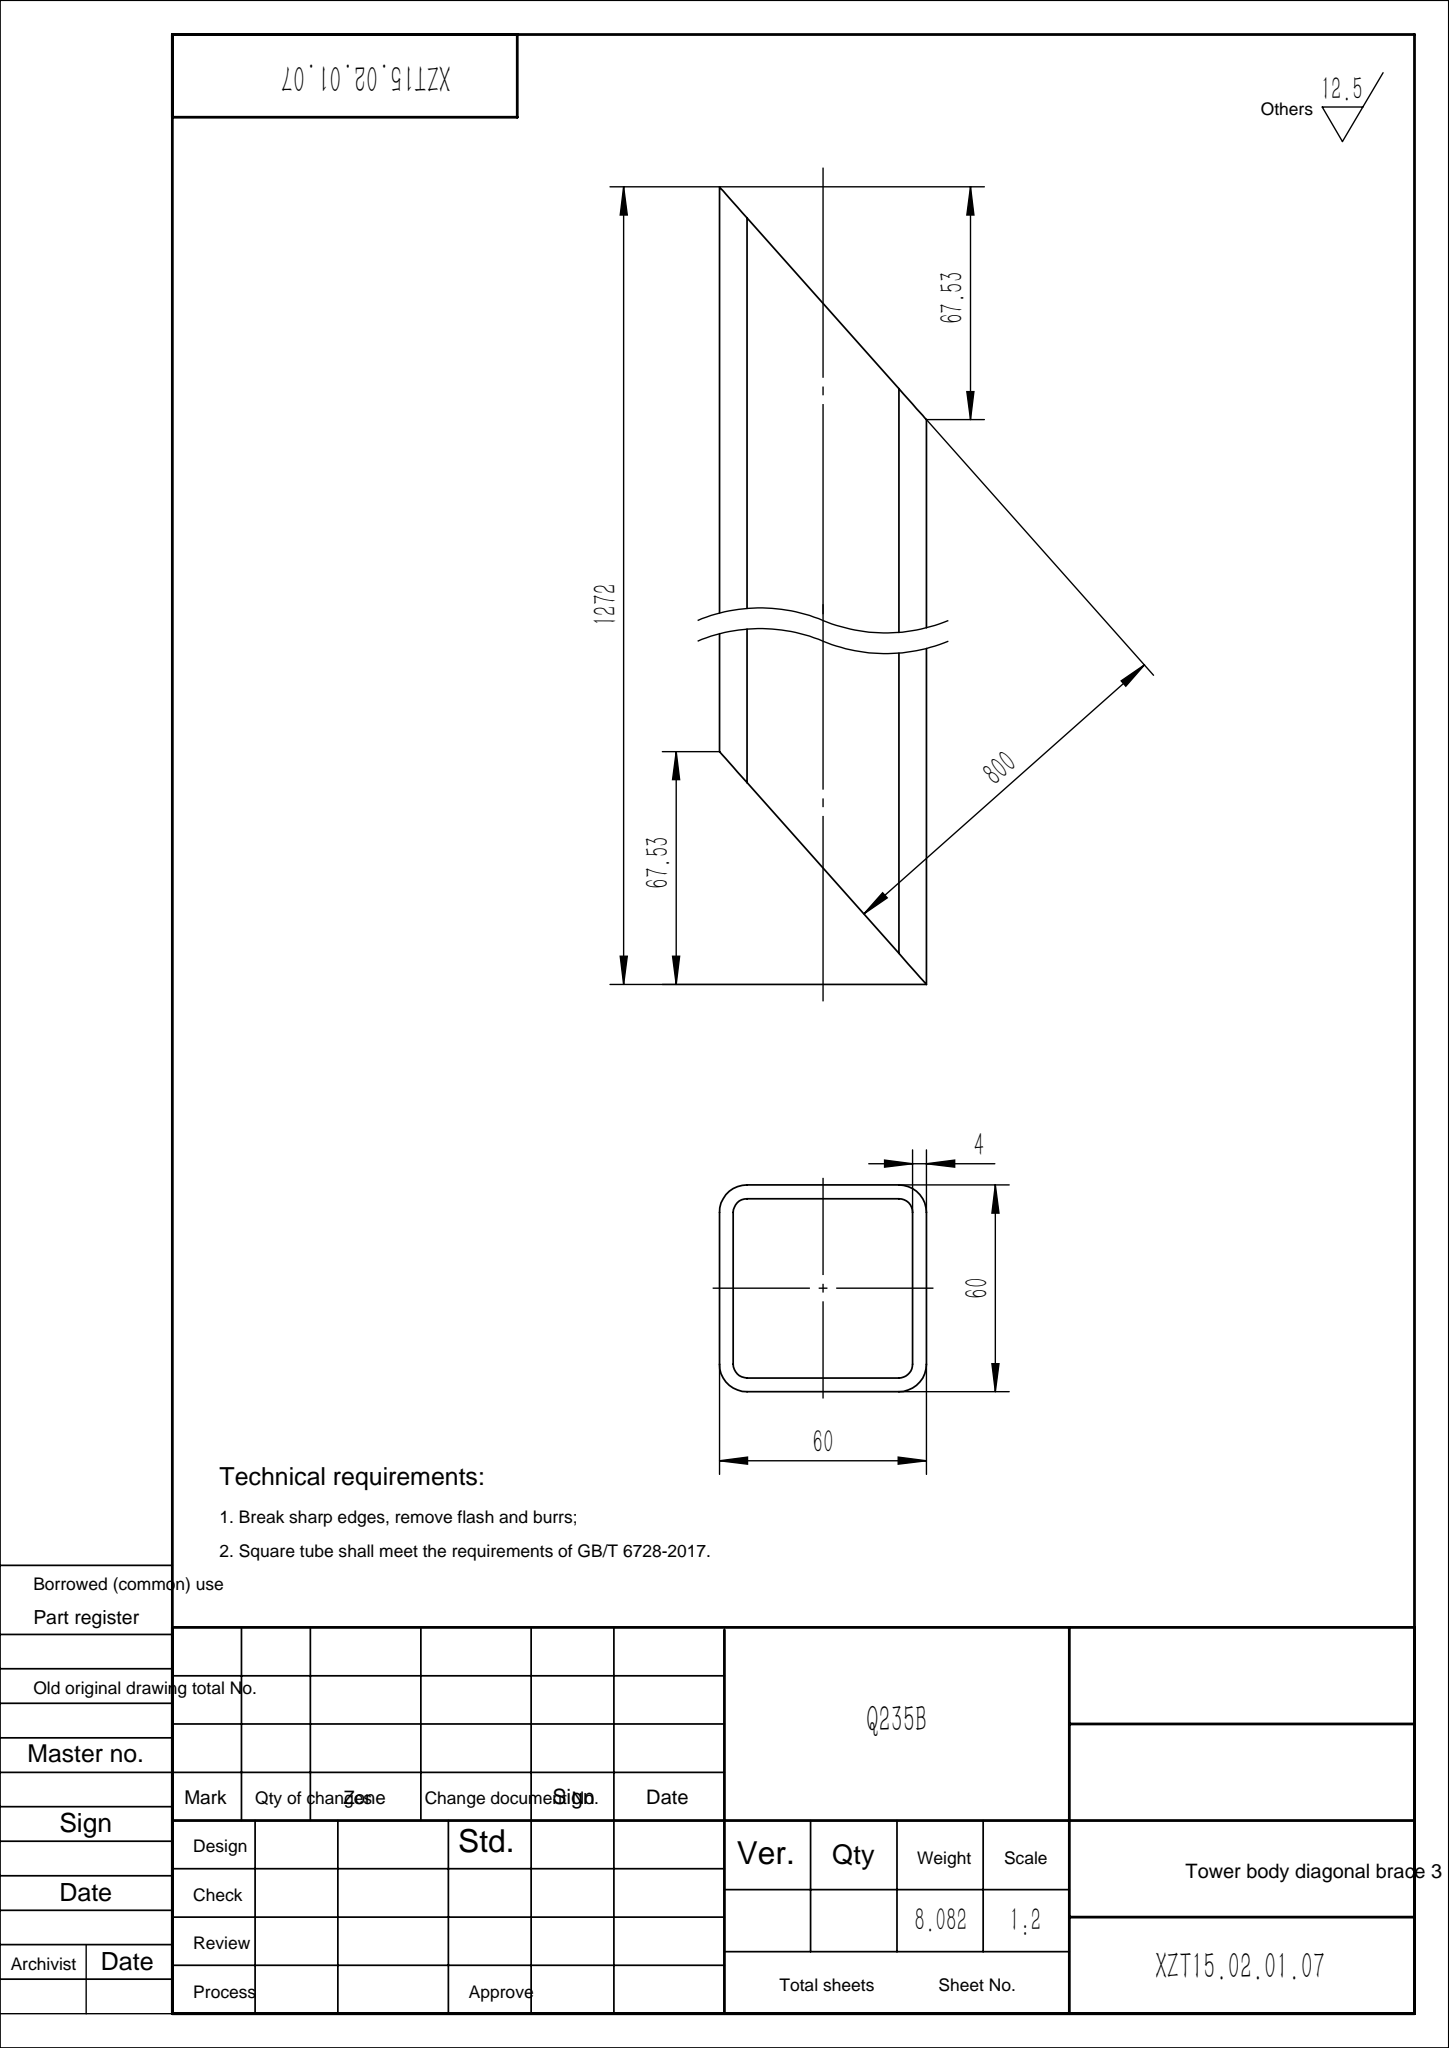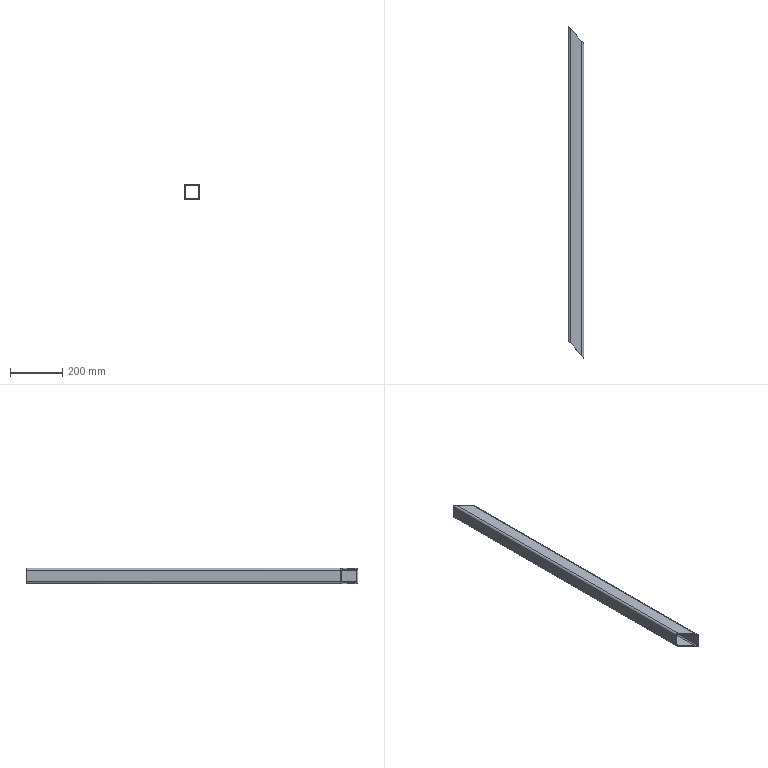Part | SolidWorks | features ICE 1, WeldMemberFeat 1, WeldmentFeature 1 | 1 solid | 18 faces | box 60 x 1272 x 60 mm | volume 1029576 mm3 | plane 10 | cylinder 8 | commonest cylinder face diameters 8 x4 16 x4
STEP:
#1=CARTESIAN_POINT('',(30.,1204.469,-22.));
#2=VERTEX_POINT('',#1);
#3=CARTESIAN_POINT('',(30.,0.,-22.));
#4=VERTEX_POINT('',#3);
#5=CARTESIAN_POINT('',(30.,1272.,-22.));
#6=DIRECTION('',(0.,-1.,0.));
#7=VECTOR('',#6,1000.);
#8=LINE('',#5,#7);
#9=EDGE_CURVE('',#2,#4,#8,.T.);
#10=ORIENTED_EDGE('',*,*,#9,.F.);
#11=CARTESIAN_POINT('',(30.,1204.469,22.));
#12=VERTEX_POINT('',#11);
#13=CARTESIAN_POINT('',(30.,1204.469,-30.));
#14=DIRECTION('',(0.,0.,1.));
#15=VECTOR('',#14,1000.);
#16=LINE('',#13,#15);
#17=EDGE_CURVE('',#2,#12,#16,.T.);
#18=ORIENTED_EDGE('',*,*,#17,.T.);
#19=CARTESIAN_POINT('',(30.,0.,22.));
#20=VERTEX_POINT('',#19);
#21=CARTESIAN_POINT('',(30.,1272.,22.));
#22=DIRECTION('',(0.,-1.,0.));
#23=VECTOR('',#22,1000.);
#24=LINE('',#21,#23);
#25=EDGE_CURVE('',#12,#20,#24,.T.);
#26=ORIENTED_EDGE('',*,*,#25,.T.);
#27=CARTESIAN_POINT('',(30.,0.,-22.));
#28=DIRECTION('',(0.,0.,-1.));
#29=VECTOR('',#28,1000.);
#30=LINE('',#27,#29);
#31=EDGE_CURVE('',#20,#4,#30,.T.);
#32=ORIENTED_EDGE('',*,*,#31,.T.);
#33=EDGE_LOOP('',(#10,#18,#26,#32));
#34=FACE_OUTER_BOUND('',#33,.T.);
#35=CARTESIAN_POINT('',(30.,1272.,-22.));
#36=DIRECTION('',(-1.,0.,0.));
#37=DIRECTION('',(0.,0.,1.));
#38=AXIS2_PLACEMENT_3D('',#35,#36,#37);
#39=PLANE('',#38);
#40=ADVANCED_FACE('',(#34),#39,.F.);
#41=CARTESIAN_POINT('',(-30.,1272.,-22.));
#42=VERTEX_POINT('',#41);
#43=CARTESIAN_POINT('',(-30.,67.531,-22.));
#44=VERTEX_POINT('',#43);
#45=CARTESIAN_POINT('',(-30.,1272.,-22.));
#46=DIRECTION('',(0.,-1.,0.));
#47=VECTOR('',#46,1000.);
#48=LINE('',#45,#47);
#49=EDGE_CURVE('',#42,#44,#48,.T.);
#50=ORIENTED_EDGE('',*,*,#49,.T.);
#51=CARTESIAN_POINT('',(-30.,67.531,22.));
#52=VERTEX_POINT('',#51);
#53=CARTESIAN_POINT('',(-30.,67.531,-30.));
#54=DIRECTION('',(0.,0.,1.));
#55=VECTOR('',#54,1000.);
#56=LINE('',#53,#55);
#57=EDGE_CURVE('',#44,#52,#56,.T.);
#58=ORIENTED_EDGE('',*,*,#57,.T.);
#59=CARTESIAN_POINT('',(-30.,1272.,22.));
#60=VERTEX_POINT('',#59);
#61=CARTESIAN_POINT('',(-30.,1272.,22.));
#62=DIRECTION('',(0.,-1.,0.));
#63=VECTOR('',#62,1000.);
#64=LINE('',#61,#63);
#65=EDGE_CURVE('',#60,#52,#64,.T.);
#66=ORIENTED_EDGE('',*,*,#65,.F.);
#67=CARTESIAN_POINT('',(-30.,1272.,22.));
#68=DIRECTION('',(0.,0.,1.));
#69=VECTOR('',#68,1000.);
#70=LINE('',#67,#69);
#71=EDGE_CURVE('',#42,#60,#70,.T.);
#72=ORIENTED_EDGE('',*,*,#71,.F.);
#73=EDGE_LOOP('',(#50,#58,#66,#72));
#74=FACE_OUTER_BOUND('',#73,.T.);
#75=CARTESIAN_POINT('',(-30.,1272.,22.));
#76=DIRECTION('',(1.,0.,0.));
#77=DIRECTION('',(0.,0.,-1.));
#78=AXIS2_PLACEMENT_3D('',#75,#76,#77);
#79=PLANE('',#78);
#80=ADVANCED_FACE('',(#74),#79,.F.);
#81=ORIENTED_EDGE('',*,*,#49,.F.);
#82=CARTESIAN_POINT('',(-22.,1262.996,-30.));
#83=VERTEX_POINT('',#82);
#84=CARTESIAN_POINT('',(-30.,1272.,-22.));
#85=CARTESIAN_POINT('',(-30.,1272.,-26.686));
#86=CARTESIAN_POINT('',(-26.686,1268.27,-30.));
#87=CARTESIAN_POINT('',(-22.,1262.996,-30.));
#88=(BOUNDED_CURVE()B_SPLINE_CURVE(3,(#84,#85,#86,#87),.UNSPECIFIED.,.F.,.F.)B_SPLINE_CURVE_WITH_KNOTS((4,4),(3.142,4.712),.UNSPECIFIED.)CURVE()GEOMETRIC_REPRESENTATION_ITEM()RATIONAL_B_SPLINE_CURVE((1.,0.8047,0.8047,1.))REPRESENTATION_ITEM(''));
#89=EDGE_CURVE('',#42,#83,#88,.T.);
#90=ORIENTED_EDGE('',*,*,#89,.T.);
#91=CARTESIAN_POINT('',(-22.,58.527,-30.));
#92=VERTEX_POINT('',#91);
#93=CARTESIAN_POINT('',(-22.,1272.,-30.));
#94=DIRECTION('',(0.,-1.,0.));
#95=VECTOR('',#94,1000.);
#96=LINE('',#93,#95);
#97=EDGE_CURVE('',#83,#92,#96,.T.);
#98=ORIENTED_EDGE('',*,*,#97,.T.);
#99=CARTESIAN_POINT('',(-22.,58.527,-30.));
#100=CARTESIAN_POINT('',(-26.686,63.801,-30.));
#101=CARTESIAN_POINT('',(-30.,67.531,-26.686));
#102=CARTESIAN_POINT('',(-30.,67.531,-22.));
#103=(BOUNDED_CURVE()B_SPLINE_CURVE(3,(#99,#100,#101,#102),.UNSPECIFIED.,.F.,.F.)B_SPLINE_CURVE_WITH_KNOTS((4,4),(1.571,3.142),.UNSPECIFIED.)CURVE()GEOMETRIC_REPRESENTATION_ITEM()RATIONAL_B_SPLINE_CURVE((1.,0.8047,0.8047,1.))REPRESENTATION_ITEM(''));
#104=EDGE_CURVE('',#92,#44,#103,.T.);
#105=ORIENTED_EDGE('',*,*,#104,.T.);
#106=EDGE_LOOP('',(#81,#90,#98,#105));
#107=FACE_OUTER_BOUND('',#106,.T.);
#108=CARTESIAN_POINT('',(-22.,1272.,-22.));
#109=DIRECTION('',(0.,-1.,0.));
#110=DIRECTION('',(0.,0.,-1.));
#111=AXIS2_PLACEMENT_3D('',#108,#109,#110);
#112=CYLINDRICAL_SURFACE('',#111,8.);
#113=ADVANCED_FACE('',(#107),#112,.T.);
#114=ORIENTED_EDGE('',*,*,#97,.F.);
#115=CARTESIAN_POINT('',(22.,1213.473,-30.));
#116=VERTEX_POINT('',#115);
#117=CARTESIAN_POINT('',(-30.,1272.,-30.));
#118=DIRECTION('',(0.6642,-0.7476,0.));
#119=VECTOR('',#118,1000.);
#120=LINE('',#117,#119);
#121=EDGE_CURVE('',#83,#116,#120,.T.);
#122=ORIENTED_EDGE('',*,*,#121,.T.);
#123=CARTESIAN_POINT('',(22.,9.004,-30.));
#124=VERTEX_POINT('',#123);
#125=CARTESIAN_POINT('',(22.,1272.,-30.));
#126=DIRECTION('',(0.,-1.,0.));
#127=VECTOR('',#126,1000.);
#128=LINE('',#125,#127);
#129=EDGE_CURVE('',#116,#124,#128,.T.);
#130=ORIENTED_EDGE('',*,*,#129,.T.);
#131=CARTESIAN_POINT('',(-30.,67.531,-30.));
#132=DIRECTION('',(-0.6642,0.7476,0.));
#133=VECTOR('',#132,1000.);
#134=LINE('',#131,#133);
#135=EDGE_CURVE('',#124,#92,#134,.T.);
#136=ORIENTED_EDGE('',*,*,#135,.T.);
#137=EDGE_LOOP('',(#114,#122,#130,#136));
#138=FACE_OUTER_BOUND('',#137,.T.);
#139=CARTESIAN_POINT('',(22.,1272.,-30.));
#140=DIRECTION('',(0.,0.,1.));
#141=DIRECTION('',(1.,0.,0.));
#142=AXIS2_PLACEMENT_3D('',#139,#140,#141);
#143=PLANE('',#142);
#144=ADVANCED_FACE('',(#138),#143,.F.);
#145=ORIENTED_EDGE('',*,*,#129,.F.);
#146=CARTESIAN_POINT('',(22.,1213.473,-30.));
#147=CARTESIAN_POINT('',(26.686,1208.199,-30.));
#148=CARTESIAN_POINT('',(30.,1204.469,-26.686));
#149=CARTESIAN_POINT('',(30.,1204.469,-22.));
#150=(BOUNDED_CURVE()B_SPLINE_CURVE(3,(#146,#147,#148,#149),.UNSPECIFIED.,.F.,.T.)B_SPLINE_CURVE_WITH_KNOTS((4,4),(4.712,6.283),.UNSPECIFIED.)CURVE()GEOMETRIC_REPRESENTATION_ITEM()RATIONAL_B_SPLINE_CURVE((1.,0.8047,0.8047,1.))REPRESENTATION_ITEM(''));
#151=EDGE_CURVE('',#116,#2,#150,.T.);
#152=ORIENTED_EDGE('',*,*,#151,.T.);
#153=ORIENTED_EDGE('',*,*,#9,.T.);
#154=CARTESIAN_POINT('',(30.,0.,-22.));
#155=CARTESIAN_POINT('',(30.,0.,-26.686));
#156=CARTESIAN_POINT('',(26.686,3.73,-30.));
#157=CARTESIAN_POINT('',(22.,9.004,-30.));
#158=(BOUNDED_CURVE()B_SPLINE_CURVE(3,(#154,#155,#156,#157),.UNSPECIFIED.,.F.,.F.)B_SPLINE_CURVE_WITH_KNOTS((4,4),(0.,1.571),.UNSPECIFIED.)CURVE()GEOMETRIC_REPRESENTATION_ITEM()RATIONAL_B_SPLINE_CURVE((1.,0.8047,0.8047,1.))REPRESENTATION_ITEM(''));
#159=EDGE_CURVE('',#4,#124,#158,.T.);
#160=ORIENTED_EDGE('',*,*,#159,.T.);
#161=EDGE_LOOP('',(#145,#152,#153,#160));
#162=FACE_OUTER_BOUND('',#161,.T.);
#163=CARTESIAN_POINT('',(22.,1272.,-22.));
#164=DIRECTION('',(0.,-1.,0.));
#165=DIRECTION('',(0.,0.,-1.));
#166=AXIS2_PLACEMENT_3D('',#163,#164,#165);
#167=CYLINDRICAL_SURFACE('',#166,8.);
#168=ADVANCED_FACE('',(#162),#167,.T.);
#169=ORIENTED_EDGE('',*,*,#25,.F.);
#170=CARTESIAN_POINT('',(22.,1213.473,30.));
#171=VERTEX_POINT('',#170);
#172=CARTESIAN_POINT('',(30.,1204.469,22.));
#173=CARTESIAN_POINT('',(30.,1204.469,26.686));
#174=CARTESIAN_POINT('',(26.686,1208.199,30.));
#175=CARTESIAN_POINT('',(22.,1213.473,30.));
#176=(BOUNDED_CURVE()B_SPLINE_CURVE(3,(#172,#173,#174,#175),.UNSPECIFIED.,.F.,.F.)B_SPLINE_CURVE_WITH_KNOTS((4,4),(0.,1.571),.UNSPECIFIED.)CURVE()GEOMETRIC_REPRESENTATION_ITEM()RATIONAL_B_SPLINE_CURVE((1.,0.8047,0.8047,1.))REPRESENTATION_ITEM(''));
#177=EDGE_CURVE('',#12,#171,#176,.T.);
#178=ORIENTED_EDGE('',*,*,#177,.T.);
#179=CARTESIAN_POINT('',(22.,9.004,30.));
#180=VERTEX_POINT('',#179);
#181=CARTESIAN_POINT('',(22.,1272.,30.));
#182=DIRECTION('',(0.,-1.,0.));
#183=VECTOR('',#182,1000.);
#184=LINE('',#181,#183);
#185=EDGE_CURVE('',#171,#180,#184,.T.);
#186=ORIENTED_EDGE('',*,*,#185,.T.);
#187=CARTESIAN_POINT('',(22.,9.004,30.));
#188=CARTESIAN_POINT('',(26.686,3.73,30.));
#189=CARTESIAN_POINT('',(30.,0.,26.686));
#190=CARTESIAN_POINT('',(30.,0.,22.));
#191=(BOUNDED_CURVE()B_SPLINE_CURVE(3,(#187,#188,#189,#190),.UNSPECIFIED.,.F.,.F.)B_SPLINE_CURVE_WITH_KNOTS((4,4),(4.712,6.283),.UNSPECIFIED.)CURVE()GEOMETRIC_REPRESENTATION_ITEM()RATIONAL_B_SPLINE_CURVE((1.,0.8047,0.8047,1.))REPRESENTATION_ITEM(''));
#192=EDGE_CURVE('',#180,#20,#191,.T.);
#193=ORIENTED_EDGE('',*,*,#192,.T.);
#194=EDGE_LOOP('',(#169,#178,#186,#193));
#195=FACE_OUTER_BOUND('',#194,.T.);
#196=CARTESIAN_POINT('',(22.,1272.,22.));
#197=DIRECTION('',(0.,-1.,0.));
#198=DIRECTION('',(0.,0.,-1.));
#199=AXIS2_PLACEMENT_3D('',#196,#197,#198);
#200=CYLINDRICAL_SURFACE('',#199,8.);
#201=ADVANCED_FACE('',(#195),#200,.T.);
#202=ORIENTED_EDGE('',*,*,#185,.F.);
#203=CARTESIAN_POINT('',(-22.,1262.996,30.));
#204=VERTEX_POINT('',#203);
#205=CARTESIAN_POINT('',(-26.471,1268.028,30.));
#206=DIRECTION('',(-0.6642,0.7476,0.));
#207=VECTOR('',#206,1000.);
#208=LINE('',#205,#207);
#209=EDGE_CURVE('',#171,#204,#208,.T.);
#210=ORIENTED_EDGE('',*,*,#209,.T.);
#211=CARTESIAN_POINT('',(-22.,58.527,30.));
#212=VERTEX_POINT('',#211);
#213=CARTESIAN_POINT('',(-22.,1272.,30.));
#214=DIRECTION('',(0.,-1.,0.));
#215=VECTOR('',#214,1000.);
#216=LINE('',#213,#215);
#217=EDGE_CURVE('',#204,#212,#216,.T.);
#218=ORIENTED_EDGE('',*,*,#217,.T.);
#219=CARTESIAN_POINT('',(-624.52,736.673,30.));
#220=DIRECTION('',(0.6642,-0.7476,0.));
#221=VECTOR('',#220,1000.);
#222=LINE('',#219,#221);
#223=EDGE_CURVE('',#212,#180,#222,.T.);
#224=ORIENTED_EDGE('',*,*,#223,.T.);
#225=EDGE_LOOP('',(#202,#210,#218,#224));
#226=FACE_OUTER_BOUND('',#225,.T.);
#227=CARTESIAN_POINT('',(-22.,1272.,30.));
#228=DIRECTION('',(0.,0.,-1.));
#229=DIRECTION('',(-1.,0.,0.));
#230=AXIS2_PLACEMENT_3D('',#227,#228,#229);
#231=PLANE('',#230);
#232=ADVANCED_FACE('',(#226),#231,.F.);
#233=ORIENTED_EDGE('',*,*,#217,.F.);
#234=CARTESIAN_POINT('',(-22.,1262.996,30.));
#235=CARTESIAN_POINT('',(-26.686,1268.27,30.));
#236=CARTESIAN_POINT('',(-30.,1272.,26.686));
#237=CARTESIAN_POINT('',(-30.,1272.,22.));
#238=(BOUNDED_CURVE()B_SPLINE_CURVE(3,(#234,#235,#236,#237),.UNSPECIFIED.,.F.,.F.)B_SPLINE_CURVE_WITH_KNOTS((4,4),(1.571,3.142),.UNSPECIFIED.)CURVE()GEOMETRIC_REPRESENTATION_ITEM()RATIONAL_B_SPLINE_CURVE((1.,0.8047,0.8047,1.))REPRESENTATION_ITEM(''));
#239=EDGE_CURVE('',#204,#60,#238,.T.);
#240=ORIENTED_EDGE('',*,*,#239,.T.);
#241=ORIENTED_EDGE('',*,*,#65,.T.);
#242=CARTESIAN_POINT('',(-30.,67.531,22.));
#243=CARTESIAN_POINT('',(-30.,67.531,26.686));
#244=CARTESIAN_POINT('',(-26.686,63.801,30.));
#245=CARTESIAN_POINT('',(-22.,58.527,30.));
#246=(BOUNDED_CURVE()B_SPLINE_CURVE(3,(#242,#243,#244,#245),.UNSPECIFIED.,.F.,.F.)B_SPLINE_CURVE_WITH_KNOTS((4,4),(3.142,4.712),.UNSPECIFIED.)CURVE()GEOMETRIC_REPRESENTATION_ITEM()RATIONAL_B_SPLINE_CURVE((1.,0.8047,0.8047,1.))REPRESENTATION_ITEM(''));
#247=EDGE_CURVE('',#52,#212,#246,.T.);
#248=ORIENTED_EDGE('',*,*,#247,.T.);
#249=EDGE_LOOP('',(#233,#240,#241,#248));
#250=FACE_OUTER_BOUND('',#249,.T.);
#251=CARTESIAN_POINT('',(-22.,1272.,22.));
#252=DIRECTION('',(0.,-1.,0.));
#253=DIRECTION('',(0.,0.,-1.));
#254=AXIS2_PLACEMENT_3D('',#251,#252,#253);
#255=CYLINDRICAL_SURFACE('',#254,8.);
#256=ADVANCED_FACE('',(#250),#255,.T.);
#257=CARTESIAN_POINT('',(22.,9.004,26.));
#258=VERTEX_POINT('',#257);
#259=CARTESIAN_POINT('',(26.,4.502,22.));
#260=VERTEX_POINT('',#259);
#261=CARTESIAN_POINT('',(22.,9.004,26.));
#262=CARTESIAN_POINT('',(24.343,6.367,26.));
#263=CARTESIAN_POINT('',(26.,4.502,24.343));
#264=CARTESIAN_POINT('',(26.,4.502,22.));
#265=(BOUNDED_CURVE()B_SPLINE_CURVE(3,(#261,#262,#263,#264),.UNSPECIFIED.,.F.,.F.)B_SPLINE_CURVE_WITH_KNOTS((4,4),(4.712,6.283),.UNSPECIFIED.)CURVE()GEOMETRIC_REPRESENTATION_ITEM()RATIONAL_B_SPLINE_CURVE((1.,0.8047,0.8047,1.))REPRESENTATION_ITEM(''));
#266=EDGE_CURVE('',#258,#260,#265,.T.);
#267=ORIENTED_EDGE('',*,*,#266,.T.);
#268=CARTESIAN_POINT('',(26.,4.502,-22.));
#269=VERTEX_POINT('',#268);
#270=CARTESIAN_POINT('',(26.,4.502,-22.));
#271=DIRECTION('',(0.,0.,-1.));
#272=VECTOR('',#271,1000.);
#273=LINE('',#270,#272);
#274=EDGE_CURVE('',#260,#269,#273,.T.);
#275=ORIENTED_EDGE('',*,*,#274,.T.);
#276=CARTESIAN_POINT('',(22.,9.004,-26.));
#277=VERTEX_POINT('',#276);
#278=CARTESIAN_POINT('',(26.,4.502,-22.));
#279=CARTESIAN_POINT('',(26.,4.502,-24.343));
#280=CARTESIAN_POINT('',(24.343,6.367,-26.));
#281=CARTESIAN_POINT('',(22.,9.004,-26.));
#282=(BOUNDED_CURVE()B_SPLINE_CURVE(3,(#278,#279,#280,#281),.UNSPECIFIED.,.F.,.F.)B_SPLINE_CURVE_WITH_KNOTS((4,4),(0.,1.571),.UNSPECIFIED.)CURVE()GEOMETRIC_REPRESENTATION_ITEM()RATIONAL_B_SPLINE_CURVE((1.,0.8047,0.8047,1.))REPRESENTATION_ITEM(''));
#283=EDGE_CURVE('',#269,#277,#282,.T.);
#284=ORIENTED_EDGE('',*,*,#283,.T.);
#285=CARTESIAN_POINT('',(-22.,58.527,-26.));
#286=VERTEX_POINT('',#285);
#287=CARTESIAN_POINT('',(-605.109,714.826,-26.));
#288=DIRECTION('',(-0.6642,0.7476,0.));
#289=VECTOR('',#288,1000.);
#290=LINE('',#287,#289);
#291=EDGE_CURVE('',#277,#286,#290,.T.);
#292=ORIENTED_EDGE('',*,*,#291,.T.);
#293=CARTESIAN_POINT('',(-26.,63.029,-22.));
#294=VERTEX_POINT('',#293);
#295=CARTESIAN_POINT('',(-22.,58.527,-26.));
#296=CARTESIAN_POINT('',(-24.343,61.164,-26.));
#297=CARTESIAN_POINT('',(-26.,63.029,-24.343));
#298=CARTESIAN_POINT('',(-26.,63.029,-22.));
#299=(BOUNDED_CURVE()B_SPLINE_CURVE(3,(#295,#296,#297,#298),.UNSPECIFIED.,.F.,.F.)B_SPLINE_CURVE_WITH_KNOTS((4,4),(1.571,3.142),.UNSPECIFIED.)CURVE()GEOMETRIC_REPRESENTATION_ITEM()RATIONAL_B_SPLINE_CURVE((1.,0.8047,0.8047,1.))REPRESENTATION_ITEM(''));
#300=EDGE_CURVE('',#286,#294,#299,.T.);
#301=ORIENTED_EDGE('',*,*,#300,.T.);
#302=CARTESIAN_POINT('',(-26.,63.029,22.));
#303=VERTEX_POINT('',#302);
#304=CARTESIAN_POINT('',(-26.,63.029,22.));
#305=DIRECTION('',(0.,0.,1.));
#306=VECTOR('',#305,1000.);
#307=LINE('',#304,#306);
#308=EDGE_CURVE('',#294,#303,#307,.T.);
#309=ORIENTED_EDGE('',*,*,#308,.T.);
#310=CARTESIAN_POINT('',(-22.,58.527,26.));
#311=VERTEX_POINT('',#310);
#312=CARTESIAN_POINT('',(-26.,63.029,22.));
#313=CARTESIAN_POINT('',(-26.,63.029,24.343));
#314=CARTESIAN_POINT('',(-24.343,61.164,26.));
#315=CARTESIAN_POINT('',(-22.,58.527,26.));
#316=(BOUNDED_CURVE()B_SPLINE_CURVE(3,(#312,#313,#314,#315),.UNSPECIFIED.,.F.,.F.)B_SPLINE_CURVE_WITH_KNOTS((4,4),(3.142,4.712),.UNSPECIFIED.)CURVE()GEOMETRIC_REPRESENTATION_ITEM()RATIONAL_B_SPLINE_CURVE((1.,0.8047,0.8047,1.))REPRESENTATION_ITEM(''));
#317=EDGE_CURVE('',#303,#311,#316,.T.);
#318=ORIENTED_EDGE('',*,*,#317,.T.);
#319=CARTESIAN_POINT('',(-624.52,736.673,26.));
#320=DIRECTION('',(0.6642,-0.7476,0.));
#321=VECTOR('',#320,1000.);
#322=LINE('',#319,#321);
#323=EDGE_CURVE('',#311,#258,#322,.T.);
#324=ORIENTED_EDGE('',*,*,#323,.T.);
#325=EDGE_LOOP('',(#267,#275,#284,#292,#301,#309,#318,#324));
#326=FACE_BOUND('',#325,.T.);
#327=ORIENTED_EDGE('',*,*,#57,.F.);
#328=ORIENTED_EDGE('',*,*,#104,.F.);
#329=ORIENTED_EDGE('',*,*,#135,.F.);
#330=ORIENTED_EDGE('',*,*,#159,.F.);
#331=ORIENTED_EDGE('',*,*,#31,.F.);
#332=ORIENTED_EDGE('',*,*,#192,.F.);
#333=ORIENTED_EDGE('',*,*,#223,.F.);
#334=ORIENTED_EDGE('',*,*,#247,.F.);
#335=EDGE_LOOP('',(#327,#328,#329,#330,#331,#332,#333,#334));
#336=FACE_OUTER_BOUND('',#335,.T.);
#337=CARTESIAN_POINT('',(-30.,67.531,-30.));
#338=DIRECTION('',(0.7476,0.6642,0.));
#339=DIRECTION('',(-0.6642,0.7476,0.));
#340=AXIS2_PLACEMENT_3D('',#337,#338,#339);
#341=PLANE('',#340);
#342=ADVANCED_FACE('',(#326,#336),#341,.F.);
#343=CARTESIAN_POINT('',(26.,1208.971,22.));
#344=VERTEX_POINT('',#343);
#345=CARTESIAN_POINT('',(22.,1213.473,26.));
#346=VERTEX_POINT('',#345);
#347=CARTESIAN_POINT('',(26.,1208.971,22.));
#348=CARTESIAN_POINT('',(26.,1208.971,24.343));
#349=CARTESIAN_POINT('',(24.343,1210.836,26.));
#350=CARTESIAN_POINT('',(22.,1213.473,26.));
#351=(BOUNDED_CURVE()B_SPLINE_CURVE(3,(#347,#348,#349,#350),.UNSPECIFIED.,.F.,.F.)B_SPLINE_CURVE_WITH_KNOTS((4,4),(0.,1.571),.UNSPECIFIED.)CURVE()GEOMETRIC_REPRESENTATION_ITEM()RATIONAL_B_SPLINE_CURVE((1.,0.8047,0.8047,1.))REPRESENTATION_ITEM(''));
#352=EDGE_CURVE('',#344,#346,#351,.T.);
#353=ORIENTED_EDGE('',*,*,#352,.T.);
#354=CARTESIAN_POINT('',(-22.,1262.996,26.));
#355=VERTEX_POINT('',#354);
#356=CARTESIAN_POINT('',(-26.471,1268.028,26.));
#357=DIRECTION('',(-0.6642,0.7476,0.));
#358=VECTOR('',#357,1000.);
#359=LINE('',#356,#358);
#360=EDGE_CURVE('',#346,#355,#359,.T.);
#361=ORIENTED_EDGE('',*,*,#360,.T.);
#362=CARTESIAN_POINT('',(-26.,1267.498,22.));
#363=VERTEX_POINT('',#362);
#364=CARTESIAN_POINT('',(-22.,1262.996,26.));
#365=CARTESIAN_POINT('',(-24.343,1265.633,26.));
#366=CARTESIAN_POINT('',(-26.,1267.498,24.343));
#367=CARTESIAN_POINT('',(-26.,1267.498,22.));
#368=(BOUNDED_CURVE()B_SPLINE_CURVE(3,(#364,#365,#366,#367),.UNSPECIFIED.,.F.,.F.)B_SPLINE_CURVE_WITH_KNOTS((4,4),(1.571,3.142),.UNSPECIFIED.)CURVE()GEOMETRIC_REPRESENTATION_ITEM()RATIONAL_B_SPLINE_CURVE((1.,0.8047,0.8047,1.))REPRESENTATION_ITEM(''));
#369=EDGE_CURVE('',#355,#363,#368,.T.);
#370=ORIENTED_EDGE('',*,*,#369,.T.);
#371=CARTESIAN_POINT('',(-26.,1267.498,-22.));
#372=VERTEX_POINT('',#371);
#373=CARTESIAN_POINT('',(-26.,1267.498,22.));
#374=DIRECTION('',(0.,0.,-1.));
#375=VECTOR('',#374,1000.);
#376=LINE('',#373,#375);
#377=EDGE_CURVE('',#363,#372,#376,.T.);
#378=ORIENTED_EDGE('',*,*,#377,.T.);
#379=CARTESIAN_POINT('',(-22.,1262.996,-26.));
#380=VERTEX_POINT('',#379);
#381=CARTESIAN_POINT('',(-26.,1267.498,-22.));
#382=CARTESIAN_POINT('',(-26.,1267.498,-24.343));
#383=CARTESIAN_POINT('',(-24.343,1265.633,-26.));
#384=CARTESIAN_POINT('',(-22.,1262.996,-26.));
#385=(BOUNDED_CURVE()B_SPLINE_CURVE(3,(#381,#382,#383,#384),.UNSPECIFIED.,.F.,.F.)B_SPLINE_CURVE_WITH_KNOTS((4,4),(3.142,4.712),.UNSPECIFIED.)CURVE()GEOMETRIC_REPRESENTATION_ITEM()RATIONAL_B_SPLINE_CURVE((1.,0.8047,0.8047,1.))REPRESENTATION_ITEM(''));
#386=EDGE_CURVE('',#372,#380,#385,.T.);
#387=ORIENTED_EDGE('',*,*,#386,.T.);
#388=CARTESIAN_POINT('',(22.,1213.473,-26.));
#389=VERTEX_POINT('',#388);
#390=CARTESIAN_POINT('',(-7.06,1246.181,-26.));
#391=DIRECTION('',(0.6642,-0.7476,0.));
#392=VECTOR('',#391,1000.);
#393=LINE('',#390,#392);
#394=EDGE_CURVE('',#380,#389,#393,.T.);
#395=ORIENTED_EDGE('',*,*,#394,.T.);
#396=CARTESIAN_POINT('',(26.,1208.971,-22.));
#397=VERTEX_POINT('',#396);
#398=CARTESIAN_POINT('',(22.,1213.473,-26.));
#399=CARTESIAN_POINT('',(24.343,1210.836,-26.));
#400=CARTESIAN_POINT('',(26.,1208.971,-24.343));
#401=CARTESIAN_POINT('',(26.,1208.971,-22.));
#402=(BOUNDED_CURVE()B_SPLINE_CURVE(3,(#398,#399,#400,#401),.UNSPECIFIED.,.F.,.F.)B_SPLINE_CURVE_WITH_KNOTS((4,4),(4.712,6.283),.UNSPECIFIED.)CURVE()GEOMETRIC_REPRESENTATION_ITEM()RATIONAL_B_SPLINE_CURVE((1.,0.8047,0.8047,1.))REPRESENTATION_ITEM(''));
#403=EDGE_CURVE('',#389,#397,#402,.T.);
#404=ORIENTED_EDGE('',*,*,#403,.T.);
#405=CARTESIAN_POINT('',(26.,1208.971,-22.));
#406=DIRECTION('',(0.,0.,1.));
#407=VECTOR('',#406,1000.);
#408=LINE('',#405,#407);
#409=EDGE_CURVE('',#397,#344,#408,.T.);
#410=ORIENTED_EDGE('',*,*,#409,.T.);
#411=EDGE_LOOP('',(#353,#361,#370,#378,#387,#395,#404,#410));
#412=FACE_BOUND('',#411,.T.);
#413=ORIENTED_EDGE('',*,*,#209,.F.);
#414=ORIENTED_EDGE('',*,*,#177,.F.);
#415=ORIENTED_EDGE('',*,*,#17,.F.);
#416=ORIENTED_EDGE('',*,*,#151,.F.);
#417=ORIENTED_EDGE('',*,*,#121,.F.);
#418=ORIENTED_EDGE('',*,*,#89,.F.);
#419=ORIENTED_EDGE('',*,*,#71,.T.);
#420=ORIENTED_EDGE('',*,*,#239,.F.);
#421=EDGE_LOOP('',(#413,#414,#415,#416,#417,#418,#419,#420));
#422=FACE_OUTER_BOUND('',#421,.T.);
#423=CARTESIAN_POINT('',(-30.,1272.,-30.));
#424=DIRECTION('',(-0.7476,-0.6642,0.));
#425=DIRECTION('',(0.6642,-0.7476,0.));
#426=AXIS2_PLACEMENT_3D('',#423,#424,#425);
#427=PLANE('',#426);
#428=ADVANCED_FACE('',(#412,#422),#427,.F.);
#429=ORIENTED_EDGE('',*,*,#352,.F.);
#430=CARTESIAN_POINT('',(26.,1272.,22.));
#431=DIRECTION('',(0.,-1.,0.));
#432=VECTOR('',#431,1000.);
#433=LINE('',#430,#432);
#434=EDGE_CURVE('',#344,#260,#433,.T.);
#435=ORIENTED_EDGE('',*,*,#434,.T.);
#436=ORIENTED_EDGE('',*,*,#266,.F.);
#437=CARTESIAN_POINT('',(22.,1272.,26.));
#438=DIRECTION('',(0.,-1.,0.));
#439=VECTOR('',#438,1000.);
#440=LINE('',#437,#439);
#441=EDGE_CURVE('',#346,#258,#440,.T.);
#442=ORIENTED_EDGE('',*,*,#441,.F.);
#443=EDGE_LOOP('',(#429,#435,#436,#442));
#444=FACE_OUTER_BOUND('',#443,.T.);
#445=CARTESIAN_POINT('',(22.,1272.,22.));
#446=DIRECTION('',(0.,-1.,0.));
#447=DIRECTION('',(0.,0.,-1.));
#448=AXIS2_PLACEMENT_3D('',#445,#446,#447);
#449=CYLINDRICAL_SURFACE('',#448,4.);
#450=ADVANCED_FACE('',(#444),#449,.F.);
#451=ORIENTED_EDGE('',*,*,#360,.F.);
#452=ORIENTED_EDGE('',*,*,#441,.T.);
#453=ORIENTED_EDGE('',*,*,#323,.F.);
#454=CARTESIAN_POINT('',(-22.,1272.,26.));
#455=DIRECTION('',(0.,-1.,0.));
#456=VECTOR('',#455,1000.);
#457=LINE('',#454,#456);
#458=EDGE_CURVE('',#355,#311,#457,.T.);
#459=ORIENTED_EDGE('',*,*,#458,.F.);
#460=EDGE_LOOP('',(#451,#452,#453,#459));
#461=FACE_OUTER_BOUND('',#460,.T.);
#462=CARTESIAN_POINT('',(-22.,1272.,26.));
#463=DIRECTION('',(0.,0.,-1.));
#464=DIRECTION('',(-1.,0.,0.));
#465=AXIS2_PLACEMENT_3D('',#462,#463,#464);
#466=PLANE('',#465);
#467=ADVANCED_FACE('',(#461),#466,.T.);
#468=ORIENTED_EDGE('',*,*,#369,.F.);
#469=ORIENTED_EDGE('',*,*,#458,.T.);
#470=ORIENTED_EDGE('',*,*,#317,.F.);
#471=CARTESIAN_POINT('',(-26.,1272.,22.));
#472=DIRECTION('',(0.,-1.,0.));
#473=VECTOR('',#472,1000.);
#474=LINE('',#471,#473);
#475=EDGE_CURVE('',#363,#303,#474,.T.);
#476=ORIENTED_EDGE('',*,*,#475,.F.);
#477=EDGE_LOOP('',(#468,#469,#470,#476));
#478=FACE_OUTER_BOUND('',#477,.T.);
#479=CARTESIAN_POINT('',(-22.,1272.,22.));
#480=DIRECTION('',(0.,-1.,0.));
#481=DIRECTION('',(0.,0.,-1.));
#482=AXIS2_PLACEMENT_3D('',#479,#480,#481);
#483=CYLINDRICAL_SURFACE('',#482,4.);
#484=ADVANCED_FACE('',(#478),#483,.F.);
#485=ORIENTED_EDGE('',*,*,#377,.F.);
#486=ORIENTED_EDGE('',*,*,#475,.T.);
#487=ORIENTED_EDGE('',*,*,#308,.F.);
#488=CARTESIAN_POINT('',(-26.,1272.,-22.));
#489=DIRECTION('',(0.,-1.,0.));
#490=VECTOR('',#489,1000.);
#491=LINE('',#488,#490);
#492=EDGE_CURVE('',#372,#294,#491,.T.);
#493=ORIENTED_EDGE('',*,*,#492,.F.);
#494=EDGE_LOOP('',(#485,#486,#487,#493));
#495=FACE_OUTER_BOUND('',#494,.T.);
#496=CARTESIAN_POINT('',(-26.,1272.,22.));
#497=DIRECTION('',(1.,0.,0.));
#498=DIRECTION('',(0.,0.,-1.));
#499=AXIS2_PLACEMENT_3D('',#496,#497,#498);
#500=PLANE('',#499);
#501=ADVANCED_FACE('',(#495),#500,.T.);
#502=ORIENTED_EDGE('',*,*,#386,.F.);
#503=ORIENTED_EDGE('',*,*,#492,.T.);
#504=ORIENTED_EDGE('',*,*,#300,.F.);
#505=CARTESIAN_POINT('',(-22.,1272.,-26.));
#506=DIRECTION('',(0.,-1.,0.));
#507=VECTOR('',#506,1000.);
#508=LINE('',#505,#507);
#509=EDGE_CURVE('',#380,#286,#508,.T.);
#510=ORIENTED_EDGE('',*,*,#509,.F.);
#511=EDGE_LOOP('',(#502,#503,#504,#510));
#512=FACE_OUTER_BOUND('',#511,.T.);
#513=CARTESIAN_POINT('',(-22.,1272.,-22.));
#514=DIRECTION('',(0.,-1.,0.));
#515=DIRECTION('',(0.,0.,-1.));
#516=AXIS2_PLACEMENT_3D('',#513,#514,#515);
#517=CYLINDRICAL_SURFACE('',#516,4.);
#518=ADVANCED_FACE('',(#512),#517,.F.);
#519=ORIENTED_EDGE('',*,*,#394,.F.);
#520=ORIENTED_EDGE('',*,*,#509,.T.);
#521=ORIENTED_EDGE('',*,*,#291,.F.);
#522=CARTESIAN_POINT('',(22.,1272.,-26.));
#523=DIRECTION('',(0.,-1.,0.));
#524=VECTOR('',#523,1000.);
#525=LINE('',#522,#524);
#526=EDGE_CURVE('',#389,#277,#525,.T.);
#527=ORIENTED_EDGE('',*,*,#526,.F.);
#528=EDGE_LOOP('',(#519,#520,#521,#527));
#529=FACE_OUTER_BOUND('',#528,.T.);
#530=CARTESIAN_POINT('',(22.,1272.,-26.));
#531=DIRECTION('',(0.,0.,1.));
#532=DIRECTION('',(1.,0.,0.));
#533=AXIS2_PLACEMENT_3D('',#530,#531,#532);
#534=PLANE('',#533);
#535=ADVANCED_FACE('',(#529),#534,.T.);
#536=ORIENTED_EDGE('',*,*,#403,.F.);
#537=ORIENTED_EDGE('',*,*,#526,.T.);
#538=ORIENTED_EDGE('',*,*,#283,.F.);
#539=CARTESIAN_POINT('',(26.,1272.,-22.));
#540=DIRECTION('',(0.,-1.,0.));
#541=VECTOR('',#540,1000.);
#542=LINE('',#539,#541);
#543=EDGE_CURVE('',#397,#269,#542,.T.);
#544=ORIENTED_EDGE('',*,*,#543,.F.);
#545=EDGE_LOOP('',(#536,#537,#538,#544));
#546=FACE_OUTER_BOUND('',#545,.T.);
#547=CARTESIAN_POINT('',(22.,1272.,-22.));
#548=DIRECTION('',(0.,-1.,0.));
#549=DIRECTION('',(0.,0.,-1.));
#550=AXIS2_PLACEMENT_3D('',#547,#548,#549);
#551=CYLINDRICAL_SURFACE('',#550,4.);
#552=ADVANCED_FACE('',(#546),#551,.F.);
#553=ORIENTED_EDGE('',*,*,#409,.F.);
#554=ORIENTED_EDGE('',*,*,#543,.T.);
#555=ORIENTED_EDGE('',*,*,#274,.F.);
#556=ORIENTED_EDGE('',*,*,#434,.F.);
#557=EDGE_LOOP('',(#553,#554,#555,#556));
#558=FACE_OUTER_BOUND('',#557,.T.);
#559=CARTESIAN_POINT('',(26.,1272.,-22.));
#560=DIRECTION('',(-1.,0.,0.));
#561=DIRECTION('',(0.,0.,1.));
#562=AXIS2_PLACEMENT_3D('',#559,#560,#561);
#563=PLANE('',#562);
#564=ADVANCED_FACE('',(#558),#563,.T.);
#565=CLOSED_SHELL('',(#40,#80,#113,#144,#168,#201,#232,#256,#342,#428,#450,#467,#484,#501,#518,#535,#552,#564));
#566=MANIFOLD_SOLID_BREP('',#565);
#567=CARTESIAN_POINT('',(0.,0.,0.));
#568=DIRECTION('',(0.,0.,1.));
#569=DIRECTION('',(1.,0.,0.));
#570=AXIS2_PLACEMENT_3D('',#567,#568,#569);
#571=(LENGTH_UNIT()NAMED_UNIT(*)SI_UNIT(.MILLI.,.METRE.));
#572=UNCERTAINTY_MEASURE_WITH_UNIT(LENGTH_MEASURE(0.00001),#571,'','');
#573=(NAMED_UNIT(*)PLANE_ANGLE_UNIT()SI_UNIT($,.RADIAN.));
#574=(NAMED_UNIT(*)SI_UNIT($,.STERADIAN.)SOLID_ANGLE_UNIT());
#575=(GEOMETRIC_REPRESENTATION_CONTEXT(3)GLOBAL_UNCERTAINTY_ASSIGNED_CONTEXT((#572))GLOBAL_UNIT_ASSIGNED_CONTEXT((#571,#573,#574))REPRESENTATION_CONTEXT('',''));
#576=ADVANCED_BREP_SHAPE_REPRESENTATION('',(#566,#570),#575);